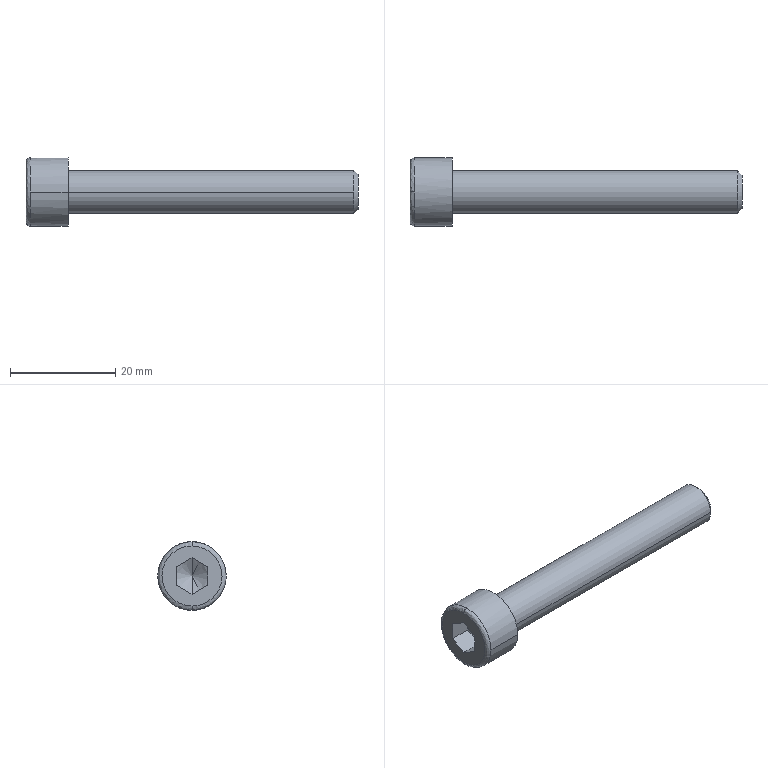Part | STEP file | AS 1420 - Metric M8 x 55 | 1 solid | 21 faces | box 63 x 13 x 13 mm | volume 3665 mm3 | plane 9 | spline 4 | cylinder 4 | cone 4 | commonest cylinder face diameters 8 x2 13 x2